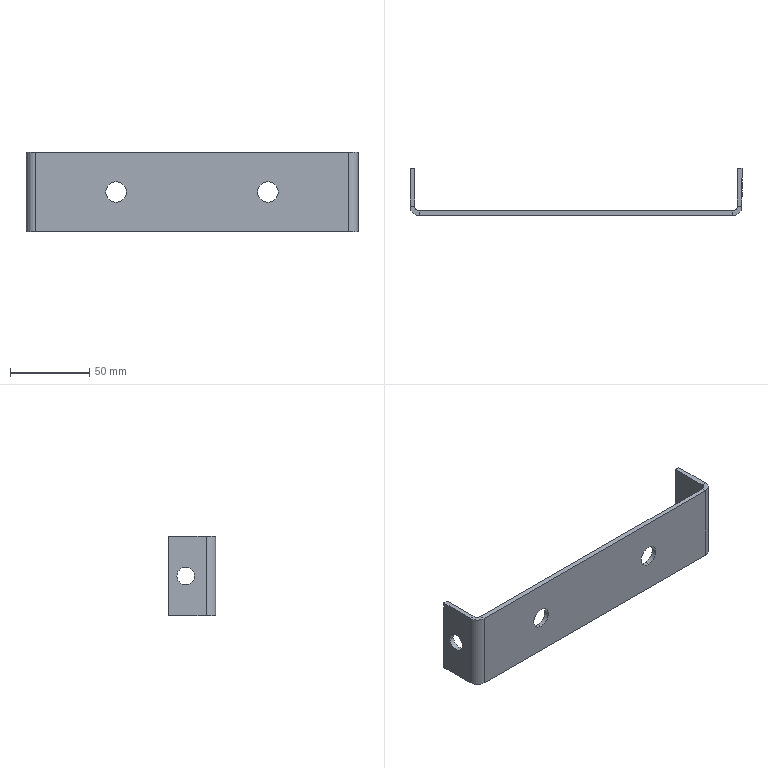Part | SolidWorks | features ICE 2, FlatPattern 1, SMBaseFlange 1, SheetMetal 1 | 1 solid | 30 faces | box 210 x 30 x 50 mm | volume 37654 mm3 | plane 18 | cylinder 12 | commonest cylinder face diameters 11 x4 13 x4 6 x2 12 x2
STEP:
#1=CARTESIAN_POINT('',(105.,24.5,0.));
#2=VERTEX_POINT('',#1);
#3=CARTESIAN_POINT('',(105.,13.5,0.));
#4=VERTEX_POINT('',#3);
#5=CARTESIAN_POINT('',(105.,19.,0.));
#6=DIRECTION('',(-1.,0.,0.));
#7=DIRECTION('',(0.,-1.,0.));
#8=AXIS2_PLACEMENT_3D('',#5,#6,#7);
#9=CIRCLE('',#8,5.5);
#10=EDGE_CURVE('',#2,#4,#9,.T.);
#11=ORIENTED_EDGE('',*,*,#10,.F.);
#12=CARTESIAN_POINT('',(102.,24.5,0.));
#13=VERTEX_POINT('',#12);
#14=CARTESIAN_POINT('',(105.,24.5,0.));
#15=DIRECTION('',(-1.,0.,0.));
#16=VECTOR('',#15,1000.);
#17=LINE('',#14,#16);
#18=EDGE_CURVE('',#2,#13,#17,.T.);
#19=ORIENTED_EDGE('',*,*,#18,.T.);
#20=CARTESIAN_POINT('',(102.,13.5,0.));
#21=VERTEX_POINT('',#20);
#22=CARTESIAN_POINT('',(102.,19.,0.));
#23=DIRECTION('',(-1.,0.,0.));
#24=DIRECTION('',(0.,-1.,0.));
#25=AXIS2_PLACEMENT_3D('',#22,#23,#24);
#26=CIRCLE('',#25,5.5);
#27=EDGE_CURVE('',#13,#21,#26,.T.);
#28=ORIENTED_EDGE('',*,*,#27,.T.);
#29=CARTESIAN_POINT('',(105.,13.5,0.));
#30=DIRECTION('',(-1.,0.,0.));
#31=VECTOR('',#30,1000.);
#32=LINE('',#29,#31);
#33=EDGE_CURVE('',#4,#21,#32,.T.);
#34=ORIENTED_EDGE('',*,*,#33,.F.);
#35=EDGE_LOOP('',(#11,#19,#28,#34));
#36=FACE_OUTER_BOUND('',#35,.T.);
#37=CARTESIAN_POINT('',(105.,19.,0.));
#38=DIRECTION('',(-1.,0.,0.));
#39=DIRECTION('',(0.,-1.,0.));
#40=AXIS2_PLACEMENT_3D('',#37,#38,#39);
#41=CYLINDRICAL_SURFACE('',#40,5.5);
#42=ADVANCED_FACE('',(#36),#41,.F.);
#43=CARTESIAN_POINT('',(-102.,13.5,0.));
#44=VERTEX_POINT('',#43);
#45=CARTESIAN_POINT('',(-102.,24.5,0.));
#46=VERTEX_POINT('',#45);
#47=CARTESIAN_POINT('',(-102.,19.,0.));
#48=DIRECTION('',(1.,0.,0.));
#49=DIRECTION('',(0.,1.,0.));
#50=AXIS2_PLACEMENT_3D('',#47,#48,#49);
#51=CIRCLE('',#50,5.5);
#52=EDGE_CURVE('',#44,#46,#51,.T.);
#53=ORIENTED_EDGE('',*,*,#52,.T.);
#54=CARTESIAN_POINT('',(-105.,24.5,0.));
#55=VERTEX_POINT('',#54);
#56=CARTESIAN_POINT('',(105.,24.5,0.));
#57=DIRECTION('',(-1.,0.,0.));
#58=VECTOR('',#57,1000.);
#59=LINE('',#56,#58);
#60=EDGE_CURVE('',#46,#55,#59,.T.);
#61=ORIENTED_EDGE('',*,*,#60,.T.);
#62=CARTESIAN_POINT('',(-105.,13.5,0.));
#63=VERTEX_POINT('',#62);
#64=CARTESIAN_POINT('',(-105.,19.,0.));
#65=DIRECTION('',(1.,0.,0.));
#66=DIRECTION('',(0.,1.,0.));
#67=AXIS2_PLACEMENT_3D('',#64,#65,#66);
#68=CIRCLE('',#67,5.5);
#69=EDGE_CURVE('',#63,#55,#68,.T.);
#70=ORIENTED_EDGE('',*,*,#69,.F.);
#71=CARTESIAN_POINT('',(105.,13.5,0.));
#72=DIRECTION('',(-1.,0.,0.));
#73=VECTOR('',#72,1000.);
#74=LINE('',#71,#73);
#75=EDGE_CURVE('',#44,#63,#74,.T.);
#76=ORIENTED_EDGE('',*,*,#75,.F.);
#77=EDGE_LOOP('',(#53,#61,#70,#76));
#78=FACE_OUTER_BOUND('',#77,.T.);
#79=CARTESIAN_POINT('',(105.,19.,0.));
#80=DIRECTION('',(-1.,0.,0.));
#81=DIRECTION('',(0.,-1.,0.));
#82=AXIS2_PLACEMENT_3D('',#79,#80,#81);
#83=CYLINDRICAL_SURFACE('',#82,5.5);
#84=ADVANCED_FACE('',(#78),#83,.F.);
#85=CARTESIAN_POINT('',(-48.,3.,-6.5));
#86=VERTEX_POINT('',#85);
#87=CARTESIAN_POINT('',(-48.,3.,6.5));
#88=VERTEX_POINT('',#87);
#89=CARTESIAN_POINT('',(-48.,3.,0.));
#90=DIRECTION('',(0.,1.,0.));
#91=DIRECTION('',(0.,0.,1.));
#92=AXIS2_PLACEMENT_3D('',#89,#90,#91);
#93=CIRCLE('',#92,6.5);
#94=EDGE_CURVE('',#86,#88,#93,.T.);
#95=ORIENTED_EDGE('',*,*,#94,.T.);
#96=CARTESIAN_POINT('',(-48.,0.,6.5));
#97=VERTEX_POINT('',#96);
#98=CARTESIAN_POINT('',(-48.,10.,6.5));
#99=DIRECTION('',(0.,-1.,0.));
#100=VECTOR('',#99,1000.);
#101=LINE('',#98,#100);
#102=EDGE_CURVE('',#88,#97,#101,.T.);
#103=ORIENTED_EDGE('',*,*,#102,.T.);
#104=CARTESIAN_POINT('',(-48.,0.,-6.5));
#105=VERTEX_POINT('',#104);
#106=CARTESIAN_POINT('',(-48.,0.,0.));
#107=DIRECTION('',(0.,-1.,0.));
#108=DIRECTION('',(0.,0.,-1.));
#109=AXIS2_PLACEMENT_3D('',#106,#107,#108);
#110=CIRCLE('',#109,6.5);
#111=EDGE_CURVE('',#97,#105,#110,.T.);
#112=ORIENTED_EDGE('',*,*,#111,.T.);
#113=CARTESIAN_POINT('',(-48.,10.,-6.5));
#114=DIRECTION('',(0.,-1.,0.));
#115=VECTOR('',#114,1000.);
#116=LINE('',#113,#115);
#117=EDGE_CURVE('',#86,#105,#116,.T.);
#118=ORIENTED_EDGE('',*,*,#117,.F.);
#119=EDGE_LOOP('',(#95,#103,#112,#118));
#120=FACE_OUTER_BOUND('',#119,.T.);
#121=CARTESIAN_POINT('',(-48.,10.,0.));
#122=DIRECTION('',(0.,-1.,0.));
#123=DIRECTION('',(0.,0.,-1.));
#124=AXIS2_PLACEMENT_3D('',#121,#122,#123);
#125=CYLINDRICAL_SURFACE('',#124,6.5);
#126=ADVANCED_FACE('',(#120),#125,.F.);
#127=CARTESIAN_POINT('',(48.,3.,-6.5));
#128=VERTEX_POINT('',#127);
#129=CARTESIAN_POINT('',(48.,3.,6.5));
#130=VERTEX_POINT('',#129);
#131=CARTESIAN_POINT('',(48.,3.,0.));
#132=DIRECTION('',(0.,1.,0.));
#133=DIRECTION('',(0.,0.,1.));
#134=AXIS2_PLACEMENT_3D('',#131,#132,#133);
#135=CIRCLE('',#134,6.5);
#136=EDGE_CURVE('',#128,#130,#135,.T.);
#137=ORIENTED_EDGE('',*,*,#136,.T.);
#138=CARTESIAN_POINT('',(48.,0.,6.5));
#139=VERTEX_POINT('',#138);
#140=CARTESIAN_POINT('',(48.,10.,6.5));
#141=DIRECTION('',(0.,-1.,0.));
#142=VECTOR('',#141,1000.);
#143=LINE('',#140,#142);
#144=EDGE_CURVE('',#130,#139,#143,.T.);
#145=ORIENTED_EDGE('',*,*,#144,.T.);
#146=CARTESIAN_POINT('',(48.,0.,-6.5));
#147=VERTEX_POINT('',#146);
#148=CARTESIAN_POINT('',(48.,0.,0.));
#149=DIRECTION('',(0.,-1.,0.));
#150=DIRECTION('',(0.,0.,-1.));
#151=AXIS2_PLACEMENT_3D('',#148,#149,#150);
#152=CIRCLE('',#151,6.5);
#153=EDGE_CURVE('',#139,#147,#152,.T.);
#154=ORIENTED_EDGE('',*,*,#153,.T.);
#155=CARTESIAN_POINT('',(48.,10.,-6.5));
#156=DIRECTION('',(0.,-1.,0.));
#157=VECTOR('',#156,1000.);
#158=LINE('',#155,#157);
#159=EDGE_CURVE('',#128,#147,#158,.T.);
#160=ORIENTED_EDGE('',*,*,#159,.F.);
#161=EDGE_LOOP('',(#137,#145,#154,#160));
#162=FACE_OUTER_BOUND('',#161,.T.);
#163=CARTESIAN_POINT('',(48.,10.,0.));
#164=DIRECTION('',(0.,-1.,0.));
#165=DIRECTION('',(0.,0.,-1.));
#166=AXIS2_PLACEMENT_3D('',#163,#164,#165);
#167=CYLINDRICAL_SURFACE('',#166,6.5);
#168=ADVANCED_FACE('',(#162),#167,.F.);
#169=CARTESIAN_POINT('',(-105.,6.,25.));
#170=VERTEX_POINT('',#169);
#171=CARTESIAN_POINT('',(-102.,6.,25.));
#172=VERTEX_POINT('',#171);
#173=CARTESIAN_POINT('',(-105.,6.,25.));
#174=DIRECTION('',(1.,0.,0.));
#175=VECTOR('',#174,1000.);
#176=LINE('',#173,#175);
#177=EDGE_CURVE('',#170,#172,#176,.T.);
#178=ORIENTED_EDGE('',*,*,#177,.F.);
#179=CARTESIAN_POINT('',(-99.,0.,25.));
#180=VERTEX_POINT('',#179);
#181=CARTESIAN_POINT('',(-99.,6.,25.));
#182=DIRECTION('',(0.,0.,1.));
#183=DIRECTION('',(-1.,0.,0.));
#184=AXIS2_PLACEMENT_3D('',#181,#182,#183);
#185=CIRCLE('',#184,6.);
#186=EDGE_CURVE('',#170,#180,#185,.T.);
#187=ORIENTED_EDGE('',*,*,#186,.T.);
#188=CARTESIAN_POINT('',(-99.,3.,25.));
#189=VERTEX_POINT('',#188);
#190=CARTESIAN_POINT('',(-99.,3.,25.));
#191=DIRECTION('',(0.,-1.,0.));
#192=VECTOR('',#191,1000.);
#193=LINE('',#190,#192);
#194=EDGE_CURVE('',#189,#180,#193,.T.);
#195=ORIENTED_EDGE('',*,*,#194,.F.);
#196=CARTESIAN_POINT('',(-99.,6.,25.));
#197=DIRECTION('',(0.,0.,1.));
#198=DIRECTION('',(1.,0.,0.));
#199=AXIS2_PLACEMENT_3D('',#196,#197,#198);
#200=CIRCLE('',#199,3.);
#201=EDGE_CURVE('',#172,#189,#200,.T.);
#202=ORIENTED_EDGE('',*,*,#201,.F.);
#203=EDGE_LOOP('',(#178,#187,#195,#202));
#204=FACE_OUTER_BOUND('',#203,.T.);
#205=CARTESIAN_POINT('',(-105.,6.,25.));
#206=DIRECTION('',(0.,0.,1.));
#207=DIRECTION('',(1.,0.,0.));
#208=AXIS2_PLACEMENT_3D('',#205,#206,#207);
#209=PLANE('',#208);
#210=ADVANCED_FACE('',(#204),#209,.T.);
#211=CARTESIAN_POINT('',(-105.,30.,25.));
#212=VERTEX_POINT('',#211);
#213=CARTESIAN_POINT('',(-105.,30.,25.));
#214=DIRECTION('',(0.,-1.,0.));
#215=VECTOR('',#214,1000.);
#216=LINE('',#213,#215);
#217=EDGE_CURVE('',#212,#170,#216,.T.);
#218=ORIENTED_EDGE('',*,*,#217,.T.);
#219=ORIENTED_EDGE('',*,*,#177,.T.);
#220=CARTESIAN_POINT('',(-102.,30.,25.));
#221=VERTEX_POINT('',#220);
#222=CARTESIAN_POINT('',(-102.,30.,25.));
#223=DIRECTION('',(0.,-1.,0.));
#224=VECTOR('',#223,1000.);
#225=LINE('',#222,#224);
#226=EDGE_CURVE('',#221,#172,#225,.T.);
#227=ORIENTED_EDGE('',*,*,#226,.F.);
#228=CARTESIAN_POINT('',(-105.,30.,25.));
#229=DIRECTION('',(1.,0.,0.));
#230=VECTOR('',#229,1000.);
#231=LINE('',#228,#230);
#232=EDGE_CURVE('',#212,#221,#231,.T.);
#233=ORIENTED_EDGE('',*,*,#232,.F.);
#234=EDGE_LOOP('',(#218,#219,#227,#233));
#235=FACE_OUTER_BOUND('',#234,.T.);
#236=CARTESIAN_POINT('',(-99.,3.,25.));
#237=DIRECTION('',(0.,0.,1.));
#238=DIRECTION('',(1.,0.,0.));
#239=AXIS2_PLACEMENT_3D('',#236,#237,#238);
#240=PLANE('',#239);
#241=ADVANCED_FACE('',(#235),#240,.T.);
#242=CARTESIAN_POINT('',(-99.,0.,-25.));
#243=VERTEX_POINT('',#242);
#244=CARTESIAN_POINT('',(-99.,3.,-25.));
#245=VERTEX_POINT('',#244);
#246=CARTESIAN_POINT('',(-99.,0.,-25.));
#247=DIRECTION('',(0.,1.,0.));
#248=VECTOR('',#247,1000.);
#249=LINE('',#246,#248);
#250=EDGE_CURVE('',#243,#245,#249,.T.);
#251=ORIENTED_EDGE('',*,*,#250,.F.);
#252=CARTESIAN_POINT('',(-105.,6.,-25.));
#253=VERTEX_POINT('',#252);
#254=CARTESIAN_POINT('',(-99.,6.,-25.));
#255=DIRECTION('',(0.,0.,1.));
#256=DIRECTION('',(-1.,0.,0.));
#257=AXIS2_PLACEMENT_3D('',#254,#255,#256);
#258=CIRCLE('',#257,6.);
#259=EDGE_CURVE('',#253,#243,#258,.T.);
#260=ORIENTED_EDGE('',*,*,#259,.F.);
#261=CARTESIAN_POINT('',(-102.,6.,-25.));
#262=VERTEX_POINT('',#261);
#263=CARTESIAN_POINT('',(-102.,6.,-25.));
#264=DIRECTION('',(-1.,0.,0.));
#265=VECTOR('',#264,1000.);
#266=LINE('',#263,#265);
#267=EDGE_CURVE('',#262,#253,#266,.T.);
#268=ORIENTED_EDGE('',*,*,#267,.F.);
#269=CARTESIAN_POINT('',(-99.,6.,-25.));
#270=DIRECTION('',(0.,0.,1.));
#271=DIRECTION('',(1.,0.,0.));
#272=AXIS2_PLACEMENT_3D('',#269,#270,#271);
#273=CIRCLE('',#272,3.);
#274=EDGE_CURVE('',#262,#245,#273,.T.);
#275=ORIENTED_EDGE('',*,*,#274,.T.);
#276=EDGE_LOOP('',(#251,#260,#268,#275));
#277=FACE_OUTER_BOUND('',#276,.T.);
#278=CARTESIAN_POINT('',(-99.,0.,-25.));
#279=DIRECTION('',(0.,0.,-1.));
#280=DIRECTION('',(-1.,0.,0.));
#281=AXIS2_PLACEMENT_3D('',#278,#279,#280);
#282=PLANE('',#281);
#283=ADVANCED_FACE('',(#277),#282,.T.);
#284=CARTESIAN_POINT('',(99.,0.,-25.));
#285=VERTEX_POINT('',#284);
#286=CARTESIAN_POINT('',(-105.,0.,-25.));
#287=DIRECTION('',(1.,0.,0.));
#288=VECTOR('',#287,1000.);
#289=LINE('',#286,#288);
#290=EDGE_CURVE('',#243,#285,#289,.T.);
#291=ORIENTED_EDGE('',*,*,#290,.F.);
#292=ORIENTED_EDGE('',*,*,#250,.T.);
#293=CARTESIAN_POINT('',(99.,3.,-25.));
#294=VERTEX_POINT('',#293);
#295=CARTESIAN_POINT('',(-105.,3.,-25.));
#296=DIRECTION('',(1.,0.,0.));
#297=VECTOR('',#296,1000.);
#298=LINE('',#295,#297);
#299=EDGE_CURVE('',#245,#294,#298,.T.);
#300=ORIENTED_EDGE('',*,*,#299,.T.);
#301=CARTESIAN_POINT('',(99.,3.,-25.));
#302=DIRECTION('',(0.,-1.,0.));
#303=VECTOR('',#302,1000.);
#304=LINE('',#301,#303);
#305=EDGE_CURVE('',#294,#285,#304,.T.);
#306=ORIENTED_EDGE('',*,*,#305,.T.);
#307=EDGE_LOOP('',(#291,#292,#300,#306));
#308=FACE_OUTER_BOUND('',#307,.T.);
#309=CARTESIAN_POINT('',(-102.,6.,-25.));
#310=DIRECTION('',(0.,0.,-1.));
#311=DIRECTION('',(-1.,0.,0.));
#312=AXIS2_PLACEMENT_3D('',#309,#310,#311);
#313=PLANE('',#312);
#314=ADVANCED_FACE('',(#308),#313,.T.);
#315=CARTESIAN_POINT('',(99.,0.,25.));
#316=VERTEX_POINT('',#315);
#317=CARTESIAN_POINT('',(99.,3.,25.));
#318=VERTEX_POINT('',#317);
#319=CARTESIAN_POINT('',(99.,0.,25.));
#320=DIRECTION('',(0.,1.,0.));
#321=VECTOR('',#320,1000.);
#322=LINE('',#319,#321);
#323=EDGE_CURVE('',#316,#318,#322,.T.);
#324=ORIENTED_EDGE('',*,*,#323,.F.);
#325=CARTESIAN_POINT('',(105.,6.,25.));
#326=VERTEX_POINT('',#325);
#327=CARTESIAN_POINT('',(99.,6.,25.));
#328=DIRECTION('',(0.,0.,1.));
#329=DIRECTION('',(-1.,0.,0.));
#330=AXIS2_PLACEMENT_3D('',#327,#328,#329);
#331=CIRCLE('',#330,6.);
#332=EDGE_CURVE('',#316,#326,#331,.T.);
#333=ORIENTED_EDGE('',*,*,#332,.T.);
#334=CARTESIAN_POINT('',(102.,6.,25.));
#335=VERTEX_POINT('',#334);
#336=CARTESIAN_POINT('',(102.,6.,25.));
#337=DIRECTION('',(1.,0.,0.));
#338=VECTOR('',#337,1000.);
#339=LINE('',#336,#338);
#340=EDGE_CURVE('',#335,#326,#339,.T.);
#341=ORIENTED_EDGE('',*,*,#340,.F.);
#342=CARTESIAN_POINT('',(99.,6.,25.));
#343=DIRECTION('',(0.,0.,1.));
#344=DIRECTION('',(1.,0.,0.));
#345=AXIS2_PLACEMENT_3D('',#342,#343,#344);
#346=CIRCLE('',#345,3.);
#347=EDGE_CURVE('',#318,#335,#346,.T.);
#348=ORIENTED_EDGE('',*,*,#347,.F.);
#349=EDGE_LOOP('',(#324,#333,#341,#348));
#350=FACE_OUTER_BOUND('',#349,.T.);
#351=CARTESIAN_POINT('',(99.,0.,25.));
#352=DIRECTION('',(0.,0.,1.));
#353=DIRECTION('',(1.,0.,0.));
#354=AXIS2_PLACEMENT_3D('',#351,#352,#353);
#355=PLANE('',#354);
#356=ADVANCED_FACE('',(#350),#355,.T.);
#357=CARTESIAN_POINT('',(-105.,0.,25.));
#358=DIRECTION('',(1.,0.,0.));
#359=VECTOR('',#358,1000.);
#360=LINE('',#357,#359);
#361=EDGE_CURVE('',#180,#316,#360,.T.);
#362=ORIENTED_EDGE('',*,*,#361,.T.);
#363=ORIENTED_EDGE('',*,*,#323,.T.);
#364=CARTESIAN_POINT('',(-105.,3.,25.));
#365=DIRECTION('',(1.,0.,0.));
#366=VECTOR('',#365,1000.);
#367=LINE('',#364,#366);
#368=EDGE_CURVE('',#189,#318,#367,.T.);
#369=ORIENTED_EDGE('',*,*,#368,.F.);
#370=ORIENTED_EDGE('',*,*,#194,.T.);
#371=EDGE_LOOP('',(#362,#363,#369,#370));
#372=FACE_OUTER_BOUND('',#371,.T.);
#373=CARTESIAN_POINT('',(102.,6.,25.));
#374=DIRECTION('',(0.,0.,1.));
#375=DIRECTION('',(1.,0.,0.));
#376=AXIS2_PLACEMENT_3D('',#373,#374,#375);
#377=PLANE('',#376);
#378=ADVANCED_FACE('',(#372),#377,.T.);
#379=CARTESIAN_POINT('',(105.,6.,-25.));
#380=VERTEX_POINT('',#379);
#381=CARTESIAN_POINT('',(102.,6.,-25.));
#382=VERTEX_POINT('',#381);
#383=CARTESIAN_POINT('',(105.,6.,-25.));
#384=DIRECTION('',(-1.,0.,0.));
#385=VECTOR('',#384,1000.);
#386=LINE('',#383,#385);
#387=EDGE_CURVE('',#380,#382,#386,.T.);
#388=ORIENTED_EDGE('',*,*,#387,.F.);
#389=CARTESIAN_POINT('',(99.,6.,-25.));
#390=DIRECTION('',(0.,0.,1.));
#391=DIRECTION('',(-1.,0.,0.));
#392=AXIS2_PLACEMENT_3D('',#389,#390,#391);
#393=CIRCLE('',#392,6.);
#394=EDGE_CURVE('',#285,#380,#393,.T.);
#395=ORIENTED_EDGE('',*,*,#394,.F.);
#396=ORIENTED_EDGE('',*,*,#305,.F.);
#397=CARTESIAN_POINT('',(99.,6.,-25.));
#398=DIRECTION('',(0.,0.,1.));
#399=DIRECTION('',(1.,0.,0.));
#400=AXIS2_PLACEMENT_3D('',#397,#398,#399);
#401=CIRCLE('',#400,3.);
#402=EDGE_CURVE('',#294,#382,#401,.T.);
#403=ORIENTED_EDGE('',*,*,#402,.T.);
#404=EDGE_LOOP('',(#388,#395,#396,#403));
#405=FACE_OUTER_BOUND('',#404,.T.);
#406=CARTESIAN_POINT('',(105.,6.,-25.));
#407=DIRECTION('',(0.,0.,-1.));
#408=DIRECTION('',(-1.,0.,0.));
#409=AXIS2_PLACEMENT_3D('',#406,#407,#408);
#410=PLANE('',#409);
#411=ADVANCED_FACE('',(#405),#410,.T.);
#412=CARTESIAN_POINT('',(105.,30.,-25.));
#413=VERTEX_POINT('',#412);
#414=CARTESIAN_POINT('',(105.,0.,-25.));
#415=DIRECTION('',(0.,1.,0.));
#416=VECTOR('',#415,1000.);
#417=LINE('',#414,#416);
#418=EDGE_CURVE('',#380,#413,#417,.T.);
#419=ORIENTED_EDGE('',*,*,#418,.F.);
#420=ORIENTED_EDGE('',*,*,#387,.T.);
#421=CARTESIAN_POINT('',(102.,30.,-25.));
#422=VERTEX_POINT('',#421);
#423=CARTESIAN_POINT('',(102.,0.,-25.));
#424=DIRECTION('',(0.,1.,0.));
#425=VECTOR('',#424,1000.);
#426=LINE('',#423,#425);
#427=EDGE_CURVE('',#382,#422,#426,.T.);
#428=ORIENTED_EDGE('',*,*,#427,.T.);
#429=CARTESIAN_POINT('',(102.,30.,-25.));
#430=DIRECTION('',(1.,0.,0.));
#431=VECTOR('',#430,1000.);
#432=LINE('',#429,#431);
#433=EDGE_CURVE('',#422,#413,#432,.T.);
#434=ORIENTED_EDGE('',*,*,#433,.T.);
#435=EDGE_LOOP('',(#419,#420,#428,#434));
#436=FACE_OUTER_BOUND('',#435,.T.);
#437=CARTESIAN_POINT('',(99.,3.,-25.));
#438=DIRECTION('',(0.,0.,-1.));
#439=DIRECTION('',(-1.,0.,0.));
#440=AXIS2_PLACEMENT_3D('',#437,#438,#439);
#441=PLANE('',#440);
#442=ADVANCED_FACE('',(#436),#441,.T.);
#443=CARTESIAN_POINT('',(105.,19.,0.));
#444=DIRECTION('',(-1.,0.,0.));
#445=DIRECTION('',(0.,-1.,0.));
#446=AXIS2_PLACEMENT_3D('',#443,#444,#445);
#447=CIRCLE('',#446,5.5);
#448=EDGE_CURVE('',#4,#2,#447,.T.);
#449=ORIENTED_EDGE('',*,*,#448,.T.);
#450=ORIENTED_EDGE('',*,*,#10,.T.);
#451=EDGE_LOOP('',(#449,#450));
#452=FACE_BOUND('',#451,.T.);
#453=ORIENTED_EDGE('',*,*,#418,.T.);
#454=CARTESIAN_POINT('',(105.,30.,25.));
#455=VERTEX_POINT('',#454);
#456=CARTESIAN_POINT('',(105.,30.,25.));
#457=DIRECTION('',(0.,0.,-1.));
#458=VECTOR('',#457,1000.);
#459=LINE('',#456,#458);
#460=EDGE_CURVE('',#455,#413,#459,.T.);
#461=ORIENTED_EDGE('',*,*,#460,.F.);
#462=CARTESIAN_POINT('',(105.,0.,25.));
#463=DIRECTION('',(0.,1.,0.));
#464=VECTOR('',#463,1000.);
#465=LINE('',#462,#464);
#466=EDGE_CURVE('',#326,#455,#465,.T.);
#467=ORIENTED_EDGE('',*,*,#466,.F.);
#468=CARTESIAN_POINT('',(105.,6.,25.));
#469=DIRECTION('',(0.,0.,-1.));
#470=VECTOR('',#469,1000.);
#471=LINE('',#468,#470);
#472=EDGE_CURVE('',#326,#380,#471,.T.);
#473=ORIENTED_EDGE('',*,*,#472,.T.);
#474=EDGE_LOOP('',(#453,#461,#467,#473));
#475=FACE_OUTER_BOUND('',#474,.T.);
#476=CARTESIAN_POINT('',(105.,0.,25.));
#477=DIRECTION('',(-1.,0.,0.));
#478=DIRECTION('',(0.,-1.,0.));
#479=AXIS2_PLACEMENT_3D('',#476,#477,#478);
#480=PLANE('',#479);
#481=ADVANCED_FACE('',(#452,#475),#480,.F.);
#482=ORIENTED_EDGE('',*,*,#433,.F.);
#483=CARTESIAN_POINT('',(102.,30.,25.));
#484=VERTEX_POINT('',#483);
#485=CARTESIAN_POINT('',(102.,30.,25.));
#486=DIRECTION('',(0.,0.,-1.));
#487=VECTOR('',#486,1000.);
#488=LINE('',#485,#487);
#489=EDGE_CURVE('',#484,#422,#488,.T.);
#490=ORIENTED_EDGE('',*,*,#489,.F.);
#491=CARTESIAN_POINT('',(102.,30.,25.));
#492=DIRECTION('',(1.,0.,0.));
#493=VECTOR('',#492,1000.);
#494=LINE('',#491,#493);
#495=EDGE_CURVE('',#484,#455,#494,.T.);
#496=ORIENTED_EDGE('',*,*,#495,.T.);
#497=ORIENTED_EDGE('',*,*,#460,.T.);
#498=EDGE_LOOP('',(#482,#490,#496,#497));
#499=FACE_OUTER_BOUND('',#498,.T.);
#500=CARTESIAN_POINT('',(102.,30.,25.));
#501=DIRECTION('',(0.,1.,0.));
#502=DIRECTION('',(0.,0.,1.));
#503=AXIS2_PLACEMENT_3D('',#500,#501,#502);
#504=PLANE('',#503);
#505=ADVANCED_FACE('',(#499),#504,.T.);
#506=CARTESIAN_POINT('',(102.,19.,0.));
#507=DIRECTION('',(-1.,0.,0.));
#508=DIRECTION('',(0.,-1.,0.));
#509=AXIS2_PLACEMENT_3D('',#506,#507,#508);
#510=CIRCLE('',#509,5.5);
#511=EDGE_CURVE('',#21,#13,#510,.T.);
#512=ORIENTED_EDGE('',*,*,#511,.F.);
#513=ORIENTED_EDGE('',*,*,#27,.F.);
#514=EDGE_LOOP('',(#512,#513));
#515=FACE_BOUND('',#514,.T.);
#516=ORIENTED_EDGE('',*,*,#427,.F.);
#517=CARTESIAN_POINT('',(102.,6.,25.));
#518=DIRECTION('',(0.,0.,-1.));
#519=VECTOR('',#518,1000.);
#520=LINE('',#517,#519);
#521=EDGE_CURVE('',#335,#382,#520,.T.);
#522=ORIENTED_EDGE('',*,*,#521,.F.);
#523=CARTESIAN_POINT('',(102.,0.,25.));
#524=DIRECTION('',(0.,1.,0.));
#525=VECTOR('',#524,1000.);
#526=LINE('',#523,#525);
#527=EDGE_CURVE('',#335,#484,#526,.T.);
#528=ORIENTED_EDGE('',*,*,#527,.T.);
#529=ORIENTED_EDGE('',*,*,#489,.T.);
#530=EDGE_LOOP('',(#516,#522,#528,#529));
#531=FACE_OUTER_BOUND('',#530,.T.);
#532=CARTESIAN_POINT('',(102.,0.,25.));
#533=DIRECTION('',(-1.,0.,0.));
#534=DIRECTION('',(0.,-1.,0.));
#535=AXIS2_PLACEMENT_3D('',#532,#533,#534);
#536=PLANE('',#535);
#537=ADVANCED_FACE('',(#515,#531),#536,.T.);
#538=ORIENTED_EDGE('',*,*,#402,.F.);
#539=CARTESIAN_POINT('',(99.,3.,25.));
#540=DIRECTION('',(0.,0.,-1.));
#541=VECTOR('',#540,1000.);
#542=LINE('',#539,#541);
#543=EDGE_CURVE('',#318,#294,#542,.T.);
#544=ORIENTED_EDGE('',*,*,#543,.F.);
#545=ORIENTED_EDGE('',*,*,#347,.T.);
#546=ORIENTED_EDGE('',*,*,#521,.T.);
#547=EDGE_LOOP('',(#538,#544,#545,#546));
#548=FACE_OUTER_BOUND('',#547,.T.);
#549=CARTESIAN_POINT('',(99.,6.,25.));
#550=DIRECTION('',(0.,0.,-1.));
#551=DIRECTION('',(-1.,0.,0.));
#552=AXIS2_PLACEMENT_3D('',#549,#550,#551);
#553=CYLINDRICAL_SURFACE('',#552,3.);
#554=ADVANCED_FACE('',(#548),#553,.F.);
#555=ORIENTED_EDGE('',*,*,#94,.F.);
#556=CARTESIAN_POINT('',(-48.,3.,0.));
#557=DIRECTION('',(0.,1.,0.));
#558=DIRECTION('',(0.,0.,1.));
#559=AXIS2_PLACEMENT_3D('',#556,#557,#558);
#560=CIRCLE('',#559,6.5);
#561=EDGE_CURVE('',#88,#86,#560,.T.);
#562=ORIENTED_EDGE('',*,*,#561,.F.);
#563=EDGE_LOOP('',(#555,#562));
#564=FACE_BOUND('',#563,.T.);
#565=ORIENTED_EDGE('',*,*,#136,.F.);
#566=CARTESIAN_POINT('',(48.,3.,0.));
#567=DIRECTION('',(0.,1.,0.));
#568=DIRECTION('',(0.,0.,1.));
#569=AXIS2_PLACEMENT_3D('',#566,#567,#568);
#570=CIRCLE('',#569,6.5);
#571=EDGE_CURVE('',#130,#128,#570,.T.);
#572=ORIENTED_EDGE('',*,*,#571,.F.);
#573=EDGE_LOOP('',(#565,#572));
#574=FACE_BOUND('',#573,.T.);
#575=ORIENTED_EDGE('',*,*,#299,.F.);
#576=CARTESIAN_POINT('',(-99.,3.,25.));
#577=DIRECTION('',(0.,0.,-1.));
#578=VECTOR('',#577,1000.);
#579=LINE('',#576,#578);
#580=EDGE_CURVE('',#189,#245,#579,.T.);
#581=ORIENTED_EDGE('',*,*,#580,.F.);
#582=ORIENTED_EDGE('',*,*,#368,.T.);
#583=ORIENTED_EDGE('',*,*,#543,.T.);
#584=EDGE_LOOP('',(#575,#581,#582,#583));
#585=FACE_OUTER_BOUND('',#584,.T.);
#586=CARTESIAN_POINT('',(-105.,3.,25.));
#587=DIRECTION('',(0.,1.,0.));
#588=DIRECTION('',(0.,0.,1.));
#589=AXIS2_PLACEMENT_3D('',#586,#587,#588);
#590=PLANE('',#589);
#591=ADVANCED_FACE('',(#564,#574,#585),#590,.T.);
#592=ORIENTED_EDGE('',*,*,#274,.F.);
#593=CARTESIAN_POINT('',(-102.,6.,25.));
#594=DIRECTION('',(0.,0.,-1.));
#595=VECTOR('',#594,1000.);
#596=LINE('',#593,#595);
#597=EDGE_CURVE('',#172,#262,#596,.T.);
#598=ORIENTED_EDGE('',*,*,#597,.F.);
#599=ORIENTED_EDGE('',*,*,#201,.T.);
#600=ORIENTED_EDGE('',*,*,#580,.T.);
#601=EDGE_LOOP('',(#592,#598,#599,#600));
#602=FACE_OUTER_BOUND('',#601,.T.);
#603=CARTESIAN_POINT('',(-99.,6.,25.));
#604=DIRECTION('',(0.,0.,-1.));
#605=DIRECTION('',(-1.,0.,0.));
#606=AXIS2_PLACEMENT_3D('',#603,#604,#605);
#607=CYLINDRICAL_SURFACE('',#606,3.);
#608=ADVANCED_FACE('',(#602),#607,.F.);
#609=ORIENTED_EDGE('',*,*,#52,.F.);
#610=CARTESIAN_POINT('',(-102.,19.,0.));
#611=DIRECTION('',(1.,0.,0.));
#612=DIRECTION('',(0.,1.,0.));
#613=AXIS2_PLACEMENT_3D('',#610,#611,#612);
#614=CIRCLE('',#613,5.5);
#615=EDGE_CURVE('',#46,#44,#614,.T.);
#616=ORIENTED_EDGE('',*,*,#615,.F.);
#617=EDGE_LOOP('',(#609,#616));
#618=FACE_BOUND('',#617,.T.);
#619=CARTESIAN_POINT('',(-102.,30.,-25.));
#620=VERTEX_POINT('',#619);
#621=CARTESIAN_POINT('',(-102.,30.,-25.));
#622=DIRECTION('',(0.,-1.,0.));
#623=VECTOR('',#622,1000.);
#624=LINE('',#621,#623);
#625=EDGE_CURVE('',#620,#262,#624,.T.);
#626=ORIENTED_EDGE('',*,*,#625,.F.);
#627=CARTESIAN_POINT('',(-102.,30.,25.));
#628=DIRECTION('',(0.,0.,-1.));
#629=VECTOR('',#628,1000.);
#630=LINE('',#627,#629);
#631=EDGE_CURVE('',#221,#620,#630,.T.);
#632=ORIENTED_EDGE('',*,*,#631,.F.);
#633=ORIENTED_EDGE('',*,*,#226,.T.);
#634=ORIENTED_EDGE('',*,*,#597,.T.);
#635=EDGE_LOOP('',(#626,#632,#633,#634));
#636=FACE_OUTER_BOUND('',#635,.T.);
#637=CARTESIAN_POINT('',(-102.,30.,25.));
#638=DIRECTION('',(1.,0.,0.));
#639=DIRECTION('',(0.,1.,0.));
#640=AXIS2_PLACEMENT_3D('',#637,#638,#639);
#641=PLANE('',#640);
#642=ADVANCED_FACE('',(#618,#636),#641,.T.);
#643=CARTESIAN_POINT('',(-105.,30.,-25.));
#644=VERTEX_POINT('',#643);
#645=CARTESIAN_POINT('',(-105.,30.,-25.));
#646=DIRECTION('',(1.,0.,0.));
#647=VECTOR('',#646,1000.);
#648=LINE('',#645,#647);
#649=EDGE_CURVE('',#644,#620,#648,.T.);
#650=ORIENTED_EDGE('',*,*,#649,.F.);
#651=CARTESIAN_POINT('',(-105.,30.,25.));
#652=DIRECTION('',(0.,0.,-1.));
#653=VECTOR('',#652,1000.);
#654=LINE('',#651,#653);
#655=EDGE_CURVE('',#212,#644,#654,.T.);
#656=ORIENTED_EDGE('',*,*,#655,.F.);
#657=ORIENTED_EDGE('',*,*,#232,.T.);
#658=ORIENTED_EDGE('',*,*,#631,.T.);
#659=EDGE_LOOP('',(#650,#656,#657,#658));
#660=FACE_OUTER_BOUND('',#659,.T.);
#661=CARTESIAN_POINT('',(-105.,30.,25.));
#662=DIRECTION('',(0.,1.,0.));
#663=DIRECTION('',(-1.,0.,0.));
#664=AXIS2_PLACEMENT_3D('',#661,#662,#663);
#665=PLANE('',#664);
#666=ADVANCED_FACE('',(#660),#665,.T.);
#667=ORIENTED_EDGE('',*,*,#69,.T.);
#668=CARTESIAN_POINT('',(-105.,19.,0.));
#669=DIRECTION('',(1.,0.,0.));
#670=DIRECTION('',(0.,1.,0.));
#671=AXIS2_PLACEMENT_3D('',#668,#669,#670);
#672=CIRCLE('',#671,5.5);
#673=EDGE_CURVE('',#55,#63,#672,.T.);
#674=ORIENTED_EDGE('',*,*,#673,.T.);
#675=EDGE_LOOP('',(#667,#674));
#676=FACE_BOUND('',#675,.T.);
#677=CARTESIAN_POINT('',(-105.,30.,-25.));
#678=DIRECTION('',(0.,-1.,0.));
#679=VECTOR('',#678,1000.);
#680=LINE('',#677,#679);
#681=EDGE_CURVE('',#644,#253,#680,.T.);
#682=ORIENTED_EDGE('',*,*,#681,.T.);
#683=CARTESIAN_POINT('',(-105.,6.,25.));
#684=DIRECTION('',(0.,0.,-1.));
#685=VECTOR('',#684,1000.);
#686=LINE('',#683,#685);
#687=EDGE_CURVE('',#170,#253,#686,.T.);
#688=ORIENTED_EDGE('',*,*,#687,.F.);
#689=ORIENTED_EDGE('',*,*,#217,.F.);
#690=ORIENTED_EDGE('',*,*,#655,.T.);
#691=EDGE_LOOP('',(#682,#688,#689,#690));
#692=FACE_OUTER_BOUND('',#691,.T.);
#693=CARTESIAN_POINT('',(-105.,30.,25.));
#694=DIRECTION('',(1.,0.,0.));
#695=DIRECTION('',(0.,1.,0.));
#696=AXIS2_PLACEMENT_3D('',#693,#694,#695);
#697=PLANE('',#696);
#698=ADVANCED_FACE('',(#676,#692),#697,.F.);
#699=ORIENTED_EDGE('',*,*,#259,.T.);
#700=CARTESIAN_POINT('',(-99.,0.,25.));
#701=DIRECTION('',(0.,0.,-1.));
#702=VECTOR('',#701,1000.);
#703=LINE('',#700,#702);
#704=EDGE_CURVE('',#180,#243,#703,.T.);
#705=ORIENTED_EDGE('',*,*,#704,.F.);
#706=ORIENTED_EDGE('',*,*,#186,.F.);
#707=ORIENTED_EDGE('',*,*,#687,.T.);
#708=EDGE_LOOP('',(#699,#705,#706,#707));
#709=FACE_OUTER_BOUND('',#708,.T.);
#710=CARTESIAN_POINT('',(-99.,6.,25.));
#711=DIRECTION('',(0.,0.,-1.));
#712=DIRECTION('',(-1.,0.,0.));
#713=AXIS2_PLACEMENT_3D('',#710,#711,#712);
#714=CYLINDRICAL_SURFACE('',#713,6.);
#715=ADVANCED_FACE('',(#709),#714,.T.);
#716=CARTESIAN_POINT('',(-48.,0.,0.));
#717=DIRECTION('',(0.,-1.,0.));
#718=DIRECTION('',(0.,0.,-1.));
#719=AXIS2_PLACEMENT_3D('',#716,#717,#718);
#720=CIRCLE('',#719,6.5);
#721=EDGE_CURVE('',#105,#97,#720,.T.);
#722=ORIENTED_EDGE('',*,*,#721,.F.);
#723=ORIENTED_EDGE('',*,*,#111,.F.);
#724=EDGE_LOOP('',(#722,#723));
#725=FACE_BOUND('',#724,.T.);
#726=CARTESIAN_POINT('',(48.,0.,0.));
#727=DIRECTION('',(0.,-1.,0.));
#728=DIRECTION('',(0.,0.,-1.));
#729=AXIS2_PLACEMENT_3D('',#726,#727,#728);
#730=CIRCLE('',#729,6.5);
#731=EDGE_CURVE('',#147,#139,#730,.T.);
#732=ORIENTED_EDGE('',*,*,#731,.F.);
#733=ORIENTED_EDGE('',*,*,#153,.F.);
#734=EDGE_LOOP('',(#732,#733));
#735=FACE_BOUND('',#734,.T.);
#736=ORIENTED_EDGE('',*,*,#290,.T.);
#737=CARTESIAN_POINT('',(99.,0.,25.));
#738=DIRECTION('',(0.,0.,-1.));
#739=VECTOR('',#738,1000.);
#740=LINE('',#737,#739);
#741=EDGE_CURVE('',#316,#285,#740,.T.);
#742=ORIENTED_EDGE('',*,*,#741,.F.);
#743=ORIENTED_EDGE('',*,*,#361,.F.);
#744=ORIENTED_EDGE('',*,*,#704,.T.);
#745=EDGE_LOOP('',(#736,#742,#743,#744));
#746=FACE_OUTER_BOUND('',#745,.T.);
#747=CARTESIAN_POINT('',(-105.,0.,25.));
#748=DIRECTION('',(0.,1.,0.));
#749=DIRECTION('',(0.,0.,1.));
#750=AXIS2_PLACEMENT_3D('',#747,#748,#749);
#751=PLANE('',#750);
#752=ADVANCED_FACE('',(#725,#735,#746),#751,.F.);
#753=ORIENTED_EDGE('',*,*,#394,.T.);
#754=ORIENTED_EDGE('',*,*,#472,.F.);
#755=ORIENTED_EDGE('',*,*,#332,.F.);
#756=ORIENTED_EDGE('',*,*,#741,.T.);
#757=EDGE_LOOP('',(#753,#754,#755,#756));
#758=FACE_OUTER_BOUND('',#757,.T.);
#759=CARTESIAN_POINT('',(99.,6.,25.));
#760=DIRECTION('',(0.,0.,-1.));
#761=DIRECTION('',(-1.,0.,0.));
#762=AXIS2_PLACEMENT_3D('',#759,#760,#761);
#763=CYLINDRICAL_SURFACE('',#762,6.);
#764=ADVANCED_FACE('',(#758),#763,.T.);
#765=ORIENTED_EDGE('',*,*,#466,.T.);
#766=ORIENTED_EDGE('',*,*,#495,.F.);
#767=ORIENTED_EDGE('',*,*,#527,.F.);
#768=ORIENTED_EDGE('',*,*,#340,.T.);
#769=EDGE_LOOP('',(#765,#766,#767,#768));
#770=FACE_OUTER_BOUND('',#769,.T.);
#771=CARTESIAN_POINT('',(99.,6.,25.));
#772=DIRECTION('',(0.,0.,1.));
#773=DIRECTION('',(1.,0.,0.));
#774=AXIS2_PLACEMENT_3D('',#771,#772,#773);
#775=PLANE('',#774);
#776=ADVANCED_FACE('',(#770),#775,.T.);
#777=ORIENTED_EDGE('',*,*,#625,.T.);
#778=ORIENTED_EDGE('',*,*,#267,.T.);
#779=ORIENTED_EDGE('',*,*,#681,.F.);
#780=ORIENTED_EDGE('',*,*,#649,.T.);
#781=EDGE_LOOP('',(#777,#778,#779,#780));
#782=FACE_OUTER_BOUND('',#781,.T.);
#783=CARTESIAN_POINT('',(99.,6.,-25.));
#784=DIRECTION('',(0.,0.,1.));
#785=DIRECTION('',(1.,0.,0.));
#786=AXIS2_PLACEMENT_3D('',#783,#784,#785);
#787=PLANE('',#786);
#788=ADVANCED_FACE('',(#782),#787,.F.);
#789=ORIENTED_EDGE('',*,*,#144,.F.);
#790=ORIENTED_EDGE('',*,*,#571,.T.);
#791=ORIENTED_EDGE('',*,*,#159,.T.);
#792=ORIENTED_EDGE('',*,*,#731,.T.);
#793=EDGE_LOOP('',(#789,#790,#791,#792));
#794=FACE_OUTER_BOUND('',#793,.T.);
#795=CARTESIAN_POINT('',(48.,10.,0.));
#796=DIRECTION('',(0.,-1.,0.));
#797=DIRECTION('',(0.,0.,-1.));
#798=AXIS2_PLACEMENT_3D('',#795,#796,#797);
#799=CYLINDRICAL_SURFACE('',#798,6.5);
#800=ADVANCED_FACE('',(#794),#799,.F.);
#801=ORIENTED_EDGE('',*,*,#102,.F.);
#802=ORIENTED_EDGE('',*,*,#561,.T.);
#803=ORIENTED_EDGE('',*,*,#117,.T.);
#804=ORIENTED_EDGE('',*,*,#721,.T.);
#805=EDGE_LOOP('',(#801,#802,#803,#804));
#806=FACE_OUTER_BOUND('',#805,.T.);
#807=CARTESIAN_POINT('',(-48.,10.,0.));
#808=DIRECTION('',(0.,-1.,0.));
#809=DIRECTION('',(0.,0.,-1.));
#810=AXIS2_PLACEMENT_3D('',#807,#808,#809);
#811=CYLINDRICAL_SURFACE('',#810,6.5);
#812=ADVANCED_FACE('',(#806),#811,.F.);
#813=ORIENTED_EDGE('',*,*,#60,.F.);
#814=ORIENTED_EDGE('',*,*,#615,.T.);
#815=ORIENTED_EDGE('',*,*,#75,.T.);
#816=ORIENTED_EDGE('',*,*,#673,.F.);
#817=EDGE_LOOP('',(#813,#814,#815,#816));
#818=FACE_OUTER_BOUND('',#817,.T.);
#819=CARTESIAN_POINT('',(105.,19.,0.));
#820=DIRECTION('',(-1.,0.,0.));
#821=DIRECTION('',(0.,-1.,0.));
#822=AXIS2_PLACEMENT_3D('',#819,#820,#821);
#823=CYLINDRICAL_SURFACE('',#822,5.5);
#824=ADVANCED_FACE('',(#818),#823,.F.);
#825=ORIENTED_EDGE('',*,*,#18,.F.);
#826=ORIENTED_EDGE('',*,*,#448,.F.);
#827=ORIENTED_EDGE('',*,*,#33,.T.);
#828=ORIENTED_EDGE('',*,*,#511,.T.);
#829=EDGE_LOOP('',(#825,#826,#827,#828));
#830=FACE_OUTER_BOUND('',#829,.T.);
#831=CARTESIAN_POINT('',(105.,19.,0.));
#832=DIRECTION('',(-1.,0.,0.));
#833=DIRECTION('',(0.,-1.,0.));
#834=AXIS2_PLACEMENT_3D('',#831,#832,#833);
#835=CYLINDRICAL_SURFACE('',#834,5.5);
#836=ADVANCED_FACE('',(#830),#835,.F.);
#837=CLOSED_SHELL('',(#42,#84,#126,#168,#210,#241,#283,#314,#356,#378,#411,#442,#481,#505,#537,#554,#591,#608,#642,#666,#698,#715,#752,#764,#776,#788,#800,#812,#824,#836));
#838=MANIFOLD_SOLID_BREP('',#837);
#839=CARTESIAN_POINT('',(0.,0.,0.));
#840=DIRECTION('',(0.,0.,1.));
#841=DIRECTION('',(1.,0.,0.));
#842=AXIS2_PLACEMENT_3D('',#839,#840,#841);
#843=(LENGTH_UNIT()NAMED_UNIT(*)SI_UNIT(.MILLI.,.METRE.));
#844=UNCERTAINTY_MEASURE_WITH_UNIT(LENGTH_MEASURE(0.00001),#843,'','');
#845=(NAMED_UNIT(*)PLANE_ANGLE_UNIT()SI_UNIT($,.RADIAN.));
#846=(NAMED_UNIT(*)SI_UNIT($,.STERADIAN.)SOLID_ANGLE_UNIT());
#847=(GEOMETRIC_REPRESENTATION_CONTEXT(3)GLOBAL_UNCERTAINTY_ASSIGNED_CONTEXT((#844))GLOBAL_UNIT_ASSIGNED_CONTEXT((#843,#845,#846))REPRESENTATION_CONTEXT('',''));
#848=ADVANCED_BREP_SHAPE_REPRESENTATION('',(#838,#842),#847);